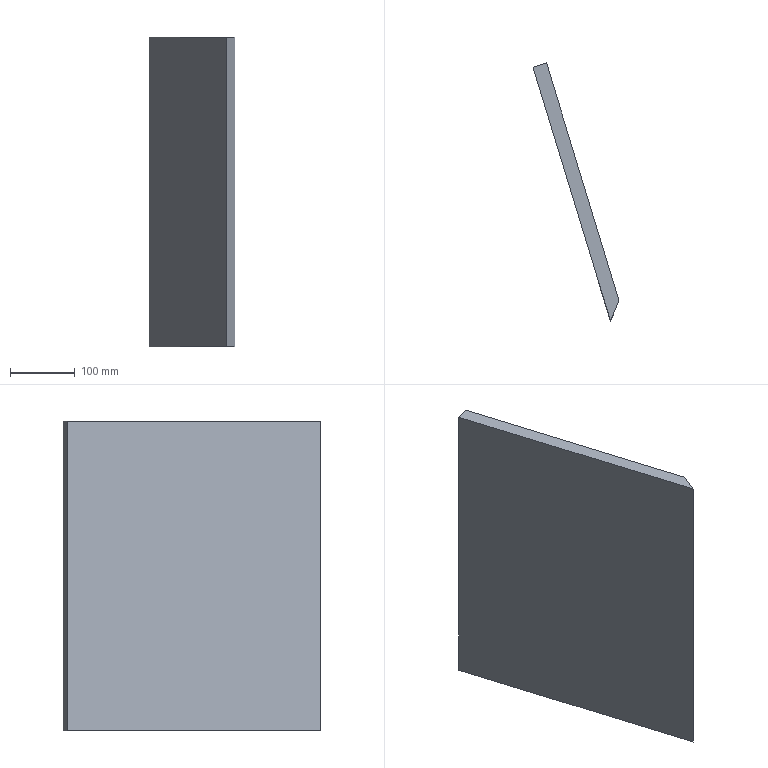Part | NX | features 底座(默认<按焊接>) 2 | 1 solid | 6 faces | box 133.231 x 399.146 x 480 mm | volume 4164554 mm3 | plane 6
STEP:
#1=CARTESIAN_POINT('',(474.285,534.59,0.));
#2=VERTEX_POINT('',#1);
#3=CARTESIAN_POINT('',(594.285,141.82,0.));
#4=VERTEX_POINT('',#3);
#5=CARTESIAN_POINT('',(1353.226,-2342.257,0.));
#6=DIRECTION('',(0.2922,-0.9564,0.));
#7=VECTOR('',#6,1000.);
#8=LINE('',#5,#7);
#9=EDGE_CURVE('',#2,#4,#8,.T.);
#10=ORIENTED_EDGE('',*,*,#9,.T.);
#11=CARTESIAN_POINT('',(594.285,141.82,480.));
#12=VERTEX_POINT('',#11);
#13=CARTESIAN_POINT('',(594.285,141.82,480.));
#14=DIRECTION('',(0.,0.,-1.));
#15=VECTOR('',#14,1000.);
#16=LINE('',#13,#15);
#17=EDGE_CURVE('',#12,#4,#16,.T.);
#18=ORIENTED_EDGE('',*,*,#17,.F.);
#19=CARTESIAN_POINT('',(474.285,534.59,480.));
#20=VERTEX_POINT('',#19);
#21=CARTESIAN_POINT('',(1353.226,-2342.257,480.));
#22=DIRECTION('',(0.2922,-0.9564,0.));
#23=VECTOR('',#22,1000.);
#24=LINE('',#21,#23);
#25=EDGE_CURVE('',#20,#12,#24,.T.);
#26=ORIENTED_EDGE('',*,*,#25,.F.);
#27=CARTESIAN_POINT('',(474.285,534.59,480.));
#28=DIRECTION('',(0.,0.,-1.));
#29=VECTOR('',#28,1000.);
#30=LINE('',#27,#29);
#31=EDGE_CURVE('',#20,#2,#30,.T.);
#32=ORIENTED_EDGE('',*,*,#31,.T.);
#33=EDGE_LOOP('',(#10,#18,#26,#32));
#34=FACE_BOUND('',#33,.T.);
#35=CARTESIAN_POINT('',(1353.226,-2342.257,480.));
#36=DIRECTION('',(0.9564,0.2922,0.));
#37=DIRECTION('',(-0.2922,0.9564,0.));
#38=AXIS2_PLACEMENT_3D('',#35,#36,#37);
#39=PLANE('',#38);
#40=ADVANCED_FACE('',(#34),#39,.F.);
#41=CARTESIAN_POINT('',(607.516,173.192,0.));
#42=VERTEX_POINT('',#41);
#43=CARTESIAN_POINT('',(-207.203,-1758.618,0.));
#44=DIRECTION('',(0.3886,0.9214,0.));
#45=VECTOR('',#44,1000.);
#46=LINE('',#43,#45);
#47=EDGE_CURVE('',#4,#42,#46,.T.);
#48=ORIENTED_EDGE('',*,*,#47,.T.);
#49=CARTESIAN_POINT('',(607.516,173.192,480.));
#50=VERTEX_POINT('',#49);
#51=CARTESIAN_POINT('',(607.516,173.192,480.));
#52=DIRECTION('',(0.,0.,-1.));
#53=VECTOR('',#52,1000.);
#54=LINE('',#51,#53);
#55=EDGE_CURVE('',#50,#42,#54,.T.);
#56=ORIENTED_EDGE('',*,*,#55,.F.);
#57=CARTESIAN_POINT('',(-207.203,-1758.618,480.));
#58=DIRECTION('',(0.3886,0.9214,0.));
#59=VECTOR('',#58,1000.);
#60=LINE('',#57,#59);
#61=EDGE_CURVE('',#12,#50,#60,.T.);
#62=ORIENTED_EDGE('',*,*,#61,.F.);
#63=ORIENTED_EDGE('',*,*,#17,.T.);
#64=EDGE_LOOP('',(#48,#56,#62,#63));
#65=FACE_BOUND('',#64,.T.);
#66=CARTESIAN_POINT('',(-207.203,-1758.618,480.));
#67=DIRECTION('',(-0.9214,0.3886,0.));
#68=DIRECTION('',(-0.3886,-0.9214,0.));
#69=AXIS2_PLACEMENT_3D('',#66,#67,#68);
#70=PLANE('',#69);
#71=ADVANCED_FACE('',(#65),#70,.F.);
#72=CARTESIAN_POINT('',(495.153,540.966,0.));
#73=VERTEX_POINT('',#72);
#74=CARTESIAN_POINT('',(1374.094,-2335.882,0.));
#75=DIRECTION('',(0.2922,-0.9564,0.));
#76=VECTOR('',#75,1000.);
#77=LINE('',#74,#76);
#78=EDGE_CURVE('',#73,#42,#77,.T.);
#79=ORIENTED_EDGE('',*,*,#78,.F.);
#80=CARTESIAN_POINT('',(495.153,540.966,480.));
#81=VERTEX_POINT('',#80);
#82=CARTESIAN_POINT('',(495.153,540.966,480.));
#83=DIRECTION('',(0.,0.,-1.));
#84=VECTOR('',#83,1000.);
#85=LINE('',#82,#84);
#86=EDGE_CURVE('',#81,#73,#85,.T.);
#87=ORIENTED_EDGE('',*,*,#86,.F.);
#88=CARTESIAN_POINT('',(1374.094,-2335.882,480.));
#89=DIRECTION('',(0.2922,-0.9564,0.));
#90=VECTOR('',#89,1000.);
#91=LINE('',#88,#90);
#92=EDGE_CURVE('',#81,#50,#91,.T.);
#93=ORIENTED_EDGE('',*,*,#92,.T.);
#94=ORIENTED_EDGE('',*,*,#55,.T.);
#95=EDGE_LOOP('',(#79,#87,#93,#94));
#96=FACE_BOUND('',#95,.T.);
#97=CARTESIAN_POINT('',(1374.094,-2335.882,480.));
#98=DIRECTION('',(0.9564,0.2922,0.));
#99=DIRECTION('',(-0.2922,0.9564,0.));
#100=AXIS2_PLACEMENT_3D('',#97,#98,#99);
#101=PLANE('',#100);
#102=ADVANCED_FACE('',(#96),#101,.T.);
#103=CARTESIAN_POINT('',(371.909,503.312,0.));
#104=DIRECTION('',(0.9564,0.2922,0.));
#105=VECTOR('',#104,1000.);
#106=LINE('',#103,#105);
#107=EDGE_CURVE('',#2,#73,#106,.T.);
#108=ORIENTED_EDGE('',*,*,#107,.F.);
#109=ORIENTED_EDGE('',*,*,#31,.F.);
#110=CARTESIAN_POINT('',(371.909,503.312,480.));
#111=DIRECTION('',(0.9564,0.2922,0.));
#112=VECTOR('',#111,1000.);
#113=LINE('',#110,#112);
#114=EDGE_CURVE('',#20,#81,#113,.T.);
#115=ORIENTED_EDGE('',*,*,#114,.T.);
#116=ORIENTED_EDGE('',*,*,#86,.T.);
#117=EDGE_LOOP('',(#108,#109,#115,#116));
#118=FACE_BOUND('',#117,.T.);
#119=CARTESIAN_POINT('',(371.909,503.312,480.));
#120=DIRECTION('',(-0.2922,0.9564,0.));
#121=DIRECTION('',(-0.9564,-0.2922,0.));
#122=AXIS2_PLACEMENT_3D('',#119,#120,#121);
#123=PLANE('',#122);
#124=ADVANCED_FACE('',(#118),#123,.T.);
#125=ORIENTED_EDGE('',*,*,#25,.T.);
#126=ORIENTED_EDGE('',*,*,#61,.T.);
#127=ORIENTED_EDGE('',*,*,#92,.F.);
#128=ORIENTED_EDGE('',*,*,#114,.F.);
#129=EDGE_LOOP('',(#125,#126,#127,#128));
#130=FACE_BOUND('',#129,.T.);
#131=CARTESIAN_POINT('',(1250.85,-2373.536,480.));
#132=DIRECTION('',(0.,0.,1.));
#133=DIRECTION('',(1.,0.,0.));
#134=AXIS2_PLACEMENT_3D('',#131,#132,#133);
#135=PLANE('',#134);
#136=ADVANCED_FACE('',(#130),#135,.T.);
#137=ORIENTED_EDGE('',*,*,#9,.F.);
#138=ORIENTED_EDGE('',*,*,#107,.T.);
#139=ORIENTED_EDGE('',*,*,#78,.T.);
#140=ORIENTED_EDGE('',*,*,#47,.F.);
#141=EDGE_LOOP('',(#137,#138,#139,#140));
#142=FACE_BOUND('',#141,.T.);
#143=CARTESIAN_POINT('',(1250.85,-2373.536,0.));
#144=DIRECTION('',(0.,0.,1.));
#145=DIRECTION('',(1.,0.,0.));
#146=AXIS2_PLACEMENT_3D('',#143,#144,#145);
#147=PLANE('',#146);
#148=ADVANCED_FACE('',(#142),#147,.F.);
#149=CLOSED_SHELL('',(#40,#71,#102,#124,#136,#148));
#150=MANIFOLD_SOLID_BREP('',#149);
#151=(LENGTH_UNIT()NAMED_UNIT(*)SI_UNIT(.MILLI.,.METRE.));
#152=UNCERTAINTY_MEASURE_WITH_UNIT(LENGTH_MEASURE(0.00001),#151,'','');
#153=(NAMED_UNIT(*)PLANE_ANGLE_UNIT()SI_UNIT($,.RADIAN.));
#154=(NAMED_UNIT(*)SI_UNIT($,.STERADIAN.)SOLID_ANGLE_UNIT());
#155=(GEOMETRIC_REPRESENTATION_CONTEXT(3)GLOBAL_UNCERTAINTY_ASSIGNED_CONTEXT((#152))GLOBAL_UNIT_ASSIGNED_CONTEXT((#151,#153,#154))REPRESENTATION_CONTEXT('',''));
#156=ADVANCED_BREP_SHAPE_REPRESENTATION('',(#150),#155);